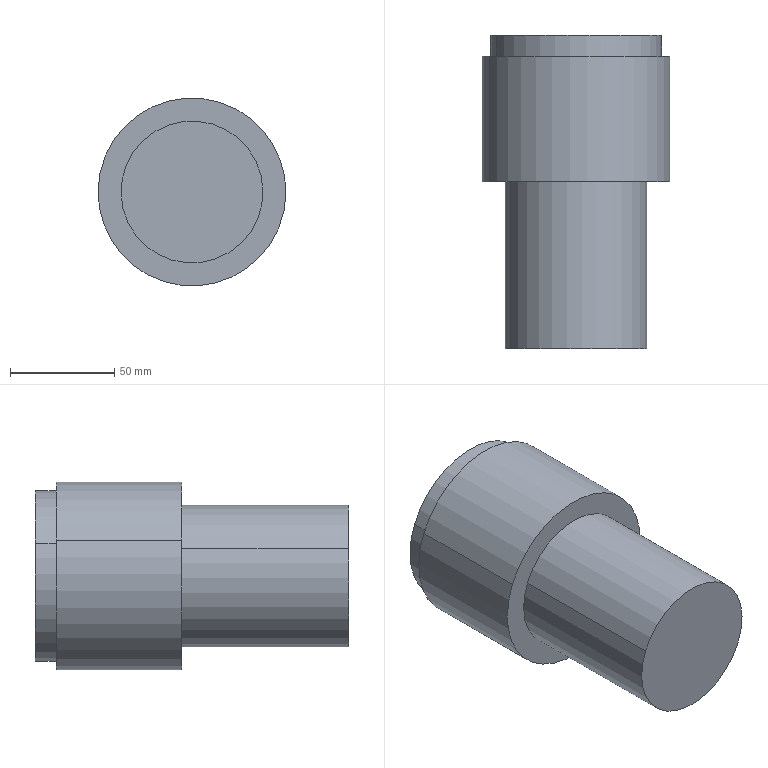Part | STEP file | Input 1-7 | 1 solid | 13 faces | box 90 x 150 x 90 mm | volume 629622 mm3 | cylinder 8 | plane 5 | commonest cylinder face diameters 45 x2 68 x2 82 x2 90 x2
STEP:
#1=CARTESIAN_POINT('',(-780.266,1724.418,3185.365));
#2=VERTEX_POINT('',#1);
#3=CARTESIAN_POINT('',(-717.452,1724.418,3159.318));
#4=VERTEX_POINT('',#3);
#5=CARTESIAN_POINT('',(-748.859,1724.418,3172.342));
#6=DIRECTION('',(0.,-1.,0.));
#7=DIRECTION('',(-0.9237,0.,0.383));
#8=AXIS2_PLACEMENT_3D('',#5,#6,#7);
#9=CIRCLE('',#8,34.);
#10=EDGE_CURVE('',#2,#4,#9,.T.);
#11=ORIENTED_EDGE('',*,*,#10,.F.);
#12=CARTESIAN_POINT('',(-780.266,1804.418,3185.365));
#13=VERTEX_POINT('',#12);
#14=CARTESIAN_POINT('',(-780.266,1724.418,3185.365));
#15=DIRECTION('',(0.,-1.,0.));
#16=VECTOR('',#15,1000.);
#17=LINE('',#14,#16);
#18=EDGE_CURVE('',#13,#2,#17,.T.);
#19=ORIENTED_EDGE('',*,*,#18,.F.);
#20=CARTESIAN_POINT('',(-717.452,1804.418,3159.318));
#21=VERTEX_POINT('',#20);
#22=CARTESIAN_POINT('',(-748.859,1804.418,3172.342));
#23=DIRECTION('',(0.,-1.,0.));
#24=DIRECTION('',(-0.9237,0.,0.383));
#25=AXIS2_PLACEMENT_3D('',#22,#23,#24);
#26=CIRCLE('',#25,34.);
#27=EDGE_CURVE('',#13,#21,#26,.T.);
#28=ORIENTED_EDGE('',*,*,#27,.T.);
#29=CARTESIAN_POINT('',(-717.452,1724.418,3159.318));
#30=DIRECTION('',(0.,-1.,0.));
#31=VECTOR('',#30,1000.);
#32=LINE('',#29,#31);
#33=EDGE_CURVE('',#21,#4,#32,.T.);
#34=ORIENTED_EDGE('',*,*,#33,.T.);
#35=EDGE_LOOP('',(#11,#19,#28,#34));
#36=FACE_OUTER_BOUND('',#35,.T.);
#37=CARTESIAN_POINT('',(-748.859,1724.418,3172.342));
#38=DIRECTION('',(0.,1.,0.));
#39=DIRECTION('',(-0.9237,0.,0.383));
#40=AXIS2_PLACEMENT_3D('',#37,#38,#39);
#41=CYLINDRICAL_SURFACE('',#40,34.);
#42=ADVANCED_FACE('',(#36),#41,.T.);
#43=CARTESIAN_POINT('',(-769.643,1814.418,3180.96));
#44=VERTEX_POINT('',#43);
#45=CARTESIAN_POINT('',(-728.075,1814.418,3163.723));
#46=VERTEX_POINT('',#45);
#47=CARTESIAN_POINT('',(-748.859,1814.418,3172.342));
#48=DIRECTION('',(0.,1.,0.));
#49=DIRECTION('',(-0.9237,0.,0.383));
#50=AXIS2_PLACEMENT_3D('',#47,#48,#49);
#51=CIRCLE('',#50,22.5);
#52=EDGE_CURVE('',#44,#46,#51,.T.);
#53=ORIENTED_EDGE('',*,*,#52,.F.);
#54=CARTESIAN_POINT('',(-769.643,1874.418,3180.96));
#55=VERTEX_POINT('',#54);
#56=CARTESIAN_POINT('',(-769.643,1724.418,3180.96));
#57=DIRECTION('',(0.,-1.,0.));
#58=VECTOR('',#57,1000.);
#59=LINE('',#56,#58);
#60=EDGE_CURVE('',#55,#44,#59,.T.);
#61=ORIENTED_EDGE('',*,*,#60,.F.);
#62=CARTESIAN_POINT('',(-728.075,1874.418,3163.723));
#63=VERTEX_POINT('',#62);
#64=CARTESIAN_POINT('',(-748.859,1874.418,3172.342));
#65=DIRECTION('',(0.,1.,0.));
#66=DIRECTION('',(0.9237,0.,-0.383));
#67=AXIS2_PLACEMENT_3D('',#64,#65,#66);
#68=CIRCLE('',#67,22.5);
#69=EDGE_CURVE('',#55,#63,#68,.T.);
#70=ORIENTED_EDGE('',*,*,#69,.T.);
#71=CARTESIAN_POINT('',(-728.075,1724.418,3163.723));
#72=DIRECTION('',(0.,-1.,0.));
#73=VECTOR('',#72,1000.);
#74=LINE('',#71,#73);
#75=EDGE_CURVE('',#63,#46,#74,.T.);
#76=ORIENTED_EDGE('',*,*,#75,.T.);
#77=EDGE_LOOP('',(#53,#61,#70,#76));
#78=FACE_OUTER_BOUND('',#77,.T.);
#79=CARTESIAN_POINT('',(-748.859,1724.418,3172.342));
#80=DIRECTION('',(0.,1.,0.));
#81=DIRECTION('',(-0.9237,0.,0.383));
#82=AXIS2_PLACEMENT_3D('',#79,#80,#81);
#83=CYLINDRICAL_SURFACE('',#82,22.5);
#84=ADVANCED_FACE('',(#78),#83,.F.);
#85=CARTESIAN_POINT('',(-710.986,1874.418,3156.637));
#86=VERTEX_POINT('',#85);
#87=CARTESIAN_POINT('',(-786.732,1874.418,3188.047));
#88=VERTEX_POINT('',#87);
#89=CARTESIAN_POINT('',(-748.859,1874.418,3172.342));
#90=DIRECTION('',(0.,1.,0.));
#91=DIRECTION('',(0.9237,0.,-0.383));
#92=AXIS2_PLACEMENT_3D('',#89,#90,#91);
#93=CIRCLE('',#92,41.);
#94=EDGE_CURVE('',#86,#88,#93,.T.);
#95=ORIENTED_EDGE('',*,*,#94,.F.);
#96=CARTESIAN_POINT('',(-710.986,1864.418,3156.637));
#97=VERTEX_POINT('',#96);
#98=CARTESIAN_POINT('',(-710.986,1874.418,3156.637));
#99=DIRECTION('',(0.,-1.,0.));
#100=VECTOR('',#99,1000.);
#101=LINE('',#98,#100);
#102=EDGE_CURVE('',#86,#97,#101,.T.);
#103=ORIENTED_EDGE('',*,*,#102,.T.);
#104=CARTESIAN_POINT('',(-786.732,1864.418,3188.047));
#105=VERTEX_POINT('',#104);
#106=CARTESIAN_POINT('',(-748.859,1864.418,3172.342));
#107=DIRECTION('',(0.,1.,0.));
#108=DIRECTION('',(-0.9237,0.,0.383));
#109=AXIS2_PLACEMENT_3D('',#106,#107,#108);
#110=CIRCLE('',#109,41.);
#111=EDGE_CURVE('',#97,#105,#110,.T.);
#112=ORIENTED_EDGE('',*,*,#111,.T.);
#113=CARTESIAN_POINT('',(-786.732,1874.418,3188.047));
#114=DIRECTION('',(0.,-1.,0.));
#115=VECTOR('',#114,1000.);
#116=LINE('',#113,#115);
#117=EDGE_CURVE('',#88,#105,#116,.T.);
#118=ORIENTED_EDGE('',*,*,#117,.F.);
#119=EDGE_LOOP('',(#95,#103,#112,#118));
#120=FACE_OUTER_BOUND('',#119,.T.);
#121=CARTESIAN_POINT('',(-748.859,1874.418,3172.342));
#122=DIRECTION('',(0.,-1.,0.));
#123=DIRECTION('',(0.9237,0.,-0.383));
#124=AXIS2_PLACEMENT_3D('',#121,#122,#123);
#125=CYLINDRICAL_SURFACE('',#124,41.);
#126=ADVANCED_FACE('',(#120),#125,.T.);
#127=CARTESIAN_POINT('',(-790.427,1804.418,3189.579));
#128=VERTEX_POINT('',#127);
#129=CARTESIAN_POINT('',(-707.291,1804.418,3155.105));
#130=VERTEX_POINT('',#129);
#131=CARTESIAN_POINT('',(-748.859,1804.418,3172.342));
#132=DIRECTION('',(0.,-1.,0.));
#133=DIRECTION('',(-0.9237,0.,0.383));
#134=AXIS2_PLACEMENT_3D('',#131,#132,#133);
#135=CIRCLE('',#134,45.);
#136=EDGE_CURVE('',#128,#130,#135,.T.);
#137=ORIENTED_EDGE('',*,*,#136,.F.);
#138=CARTESIAN_POINT('',(-790.427,1864.418,3189.579));
#139=VERTEX_POINT('',#138);
#140=CARTESIAN_POINT('',(-790.427,1814.418,3189.579));
#141=DIRECTION('',(0.,-1.,0.));
#142=VECTOR('',#141,1000.);
#143=LINE('',#140,#142);
#144=EDGE_CURVE('',#139,#128,#143,.T.);
#145=ORIENTED_EDGE('',*,*,#144,.F.);
#146=CARTESIAN_POINT('',(-707.291,1864.418,3155.105));
#147=VERTEX_POINT('',#146);
#148=CARTESIAN_POINT('',(-748.859,1864.418,3172.342));
#149=DIRECTION('',(0.,-1.,0.));
#150=DIRECTION('',(-0.9237,0.,0.383));
#151=AXIS2_PLACEMENT_3D('',#148,#149,#150);
#152=CIRCLE('',#151,45.);
#153=EDGE_CURVE('',#139,#147,#152,.T.);
#154=ORIENTED_EDGE('',*,*,#153,.T.);
#155=CARTESIAN_POINT('',(-707.291,1814.418,3155.105));
#156=DIRECTION('',(0.,-1.,0.));
#157=VECTOR('',#156,1000.);
#158=LINE('',#155,#157);
#159=EDGE_CURVE('',#147,#130,#158,.T.);
#160=ORIENTED_EDGE('',*,*,#159,.T.);
#161=EDGE_LOOP('',(#137,#145,#154,#160));
#162=FACE_OUTER_BOUND('',#161,.T.);
#163=CARTESIAN_POINT('',(-748.859,1814.418,3172.342));
#164=DIRECTION('',(0.,1.,0.));
#165=DIRECTION('',(-0.9237,0.,0.383));
#166=AXIS2_PLACEMENT_3D('',#163,#164,#165);
#167=CYLINDRICAL_SURFACE('',#166,45.);
#168=ADVANCED_FACE('',(#162),#167,.T.);
#169=CARTESIAN_POINT('',(-748.859,1804.418,3172.342));
#170=DIRECTION('',(0.,-1.,0.));
#171=DIRECTION('',(-0.9237,0.,0.383));
#172=AXIS2_PLACEMENT_3D('',#169,#170,#171);
#173=CIRCLE('',#172,45.);
#174=EDGE_CURVE('',#130,#128,#173,.T.);
#175=ORIENTED_EDGE('',*,*,#174,.T.);
#176=ORIENTED_EDGE('',*,*,#136,.T.);
#177=EDGE_LOOP('',(#175,#176));
#178=FACE_OUTER_BOUND('',#177,.T.);
#179=CARTESIAN_POINT('',(-748.859,1804.418,3172.342));
#180=DIRECTION('',(0.,-1.,0.));
#181=DIRECTION('',(-0.9237,0.,0.383));
#182=AXIS2_PLACEMENT_3D('',#179,#180,#181);
#183=CIRCLE('',#182,34.);
#184=EDGE_CURVE('',#21,#13,#183,.T.);
#185=ORIENTED_EDGE('',*,*,#184,.F.);
#186=ORIENTED_EDGE('',*,*,#27,.F.);
#187=EDGE_LOOP('',(#185,#186));
#188=FACE_BOUND('',#187,.T.);
#189=CARTESIAN_POINT('',(-748.859,1804.418,3172.342));
#190=DIRECTION('',(0.,-1.,0.));
#191=DIRECTION('',(0.9237,0.,-0.383));
#192=AXIS2_PLACEMENT_3D('',#189,#190,#191);
#193=PLANE('',#192);
#194=ADVANCED_FACE('',(#178,#188),#193,.T.);
#195=CARTESIAN_POINT('',(-748.859,1864.418,3172.342));
#196=DIRECTION('',(0.,-1.,0.));
#197=DIRECTION('',(-0.9237,0.,0.383));
#198=AXIS2_PLACEMENT_3D('',#195,#196,#197);
#199=CIRCLE('',#198,45.);
#200=EDGE_CURVE('',#147,#139,#199,.T.);
#201=ORIENTED_EDGE('',*,*,#200,.F.);
#202=ORIENTED_EDGE('',*,*,#153,.F.);
#203=EDGE_LOOP('',(#201,#202));
#204=FACE_OUTER_BOUND('',#203,.T.);
#205=CARTESIAN_POINT('',(-748.859,1864.418,3172.342));
#206=DIRECTION('',(0.,1.,0.));
#207=DIRECTION('',(-0.9237,0.,0.383));
#208=AXIS2_PLACEMENT_3D('',#205,#206,#207);
#209=CIRCLE('',#208,41.);
#210=EDGE_CURVE('',#105,#97,#209,.T.);
#211=ORIENTED_EDGE('',*,*,#210,.F.);
#212=ORIENTED_EDGE('',*,*,#111,.F.);
#213=EDGE_LOOP('',(#211,#212));
#214=FACE_BOUND('',#213,.T.);
#215=CARTESIAN_POINT('',(-748.859,1864.418,3172.342));
#216=DIRECTION('',(0.,-1.,0.));
#217=DIRECTION('',(0.9237,0.,-0.383));
#218=AXIS2_PLACEMENT_3D('',#215,#216,#217);
#219=PLANE('',#218);
#220=ADVANCED_FACE('',(#204,#214),#219,.F.);
#221=ORIENTED_EDGE('',*,*,#144,.T.);
#222=ORIENTED_EDGE('',*,*,#174,.F.);
#223=ORIENTED_EDGE('',*,*,#159,.F.);
#224=ORIENTED_EDGE('',*,*,#200,.T.);
#225=EDGE_LOOP('',(#221,#222,#223,#224));
#226=FACE_OUTER_BOUND('',#225,.T.);
#227=CARTESIAN_POINT('',(-748.859,1814.418,3172.342));
#228=DIRECTION('',(0.,1.,0.));
#229=DIRECTION('',(-0.9237,0.,0.383));
#230=AXIS2_PLACEMENT_3D('',#227,#228,#229);
#231=CYLINDRICAL_SURFACE('',#230,45.);
#232=ADVANCED_FACE('',(#226),#231,.T.);
#233=ORIENTED_EDGE('',*,*,#102,.F.);
#234=CARTESIAN_POINT('',(-748.859,1874.418,3172.342));
#235=DIRECTION('',(0.,1.,0.));
#236=DIRECTION('',(0.9237,0.,-0.383));
#237=AXIS2_PLACEMENT_3D('',#234,#235,#236);
#238=CIRCLE('',#237,41.);
#239=EDGE_CURVE('',#88,#86,#238,.T.);
#240=ORIENTED_EDGE('',*,*,#239,.F.);
#241=ORIENTED_EDGE('',*,*,#117,.T.);
#242=ORIENTED_EDGE('',*,*,#210,.T.);
#243=EDGE_LOOP('',(#233,#240,#241,#242));
#244=FACE_OUTER_BOUND('',#243,.T.);
#245=CARTESIAN_POINT('',(-748.859,1874.418,3172.342));
#246=DIRECTION('',(0.,-1.,0.));
#247=DIRECTION('',(0.9237,0.,-0.383));
#248=AXIS2_PLACEMENT_3D('',#245,#246,#247);
#249=CYLINDRICAL_SURFACE('',#248,41.);
#250=ADVANCED_FACE('',(#244),#249,.T.);
#251=CARTESIAN_POINT('',(-748.859,1874.418,3172.342));
#252=DIRECTION('',(0.,1.,0.));
#253=DIRECTION('',(0.9237,0.,-0.383));
#254=AXIS2_PLACEMENT_3D('',#251,#252,#253);
#255=CIRCLE('',#254,22.5);
#256=EDGE_CURVE('',#63,#55,#255,.T.);
#257=ORIENTED_EDGE('',*,*,#256,.F.);
#258=ORIENTED_EDGE('',*,*,#69,.F.);
#259=EDGE_LOOP('',(#257,#258));
#260=FACE_BOUND('',#259,.T.);
#261=ORIENTED_EDGE('',*,*,#239,.T.);
#262=ORIENTED_EDGE('',*,*,#94,.T.);
#263=EDGE_LOOP('',(#261,#262));
#264=FACE_OUTER_BOUND('',#263,.T.);
#265=CARTESIAN_POINT('',(-748.859,1874.418,3172.342));
#266=DIRECTION('',(0.,1.,0.));
#267=DIRECTION('',(-0.9237,0.,0.383));
#268=AXIS2_PLACEMENT_3D('',#265,#266,#267);
#269=PLANE('',#268);
#270=ADVANCED_FACE('',(#260,#264),#269,.T.);
#271=ORIENTED_EDGE('',*,*,#60,.T.);
#272=CARTESIAN_POINT('',(-748.859,1814.418,3172.342));
#273=DIRECTION('',(0.,1.,0.));
#274=DIRECTION('',(-0.9237,0.,0.383));
#275=AXIS2_PLACEMENT_3D('',#272,#273,#274);
#276=CIRCLE('',#275,22.5);
#277=EDGE_CURVE('',#46,#44,#276,.T.);
#278=ORIENTED_EDGE('',*,*,#277,.F.);
#279=ORIENTED_EDGE('',*,*,#75,.F.);
#280=ORIENTED_EDGE('',*,*,#256,.T.);
#281=EDGE_LOOP('',(#271,#278,#279,#280));
#282=FACE_OUTER_BOUND('',#281,.T.);
#283=CARTESIAN_POINT('',(-748.859,1724.418,3172.342));
#284=DIRECTION('',(0.,1.,0.));
#285=DIRECTION('',(-0.9237,0.,0.383));
#286=AXIS2_PLACEMENT_3D('',#283,#284,#285);
#287=CYLINDRICAL_SURFACE('',#286,22.5);
#288=ADVANCED_FACE('',(#282),#287,.F.);
#289=ORIENTED_EDGE('',*,*,#277,.T.);
#290=ORIENTED_EDGE('',*,*,#52,.T.);
#291=EDGE_LOOP('',(#289,#290));
#292=FACE_OUTER_BOUND('',#291,.T.);
#293=CARTESIAN_POINT('',(-748.859,1814.418,3172.342));
#294=DIRECTION('',(0.,-1.,0.));
#295=DIRECTION('',(0.9237,0.,-0.383));
#296=AXIS2_PLACEMENT_3D('',#293,#294,#295);
#297=PLANE('',#296);
#298=ADVANCED_FACE('',(#292),#297,.F.);
#299=ORIENTED_EDGE('',*,*,#18,.T.);
#300=CARTESIAN_POINT('',(-748.859,1724.418,3172.342));
#301=DIRECTION('',(0.,-1.,0.));
#302=DIRECTION('',(-0.9237,0.,0.383));
#303=AXIS2_PLACEMENT_3D('',#300,#301,#302);
#304=CIRCLE('',#303,34.);
#305=EDGE_CURVE('',#4,#2,#304,.T.);
#306=ORIENTED_EDGE('',*,*,#305,.F.);
#307=ORIENTED_EDGE('',*,*,#33,.F.);
#308=ORIENTED_EDGE('',*,*,#184,.T.);
#309=EDGE_LOOP('',(#299,#306,#307,#308));
#310=FACE_OUTER_BOUND('',#309,.T.);
#311=CARTESIAN_POINT('',(-748.859,1724.418,3172.342));
#312=DIRECTION('',(0.,1.,0.));
#313=DIRECTION('',(-0.9237,0.,0.383));
#314=AXIS2_PLACEMENT_3D('',#311,#312,#313);
#315=CYLINDRICAL_SURFACE('',#314,34.);
#316=ADVANCED_FACE('',(#310),#315,.T.);
#317=ORIENTED_EDGE('',*,*,#305,.T.);
#318=ORIENTED_EDGE('',*,*,#10,.T.);
#319=EDGE_LOOP('',(#317,#318));
#320=FACE_OUTER_BOUND('',#319,.T.);
#321=CARTESIAN_POINT('',(-748.859,1724.418,3172.342));
#322=DIRECTION('',(0.,-1.,0.));
#323=DIRECTION('',(0.9237,0.,-0.383));
#324=AXIS2_PLACEMENT_3D('',#321,#322,#323);
#325=PLANE('',#324);
#326=ADVANCED_FACE('',(#320),#325,.T.);
#327=CLOSED_SHELL('',(#42,#84,#126,#168,#194,#220,#232,#250,#270,#288,#298,#316,#326));
#328=MANIFOLD_SOLID_BREP('',#327);
#329=CARTESIAN_POINT('',(0.,0.,0.));
#330=DIRECTION('',(0.,0.,1.));
#331=DIRECTION('',(1.,0.,0.));
#332=AXIS2_PLACEMENT_3D('',#329,#330,#331);
#333=(LENGTH_UNIT()NAMED_UNIT(*)SI_UNIT(.MILLI.,.METRE.));
#334=UNCERTAINTY_MEASURE_WITH_UNIT(LENGTH_MEASURE(0.00001),#333,'','');
#335=(NAMED_UNIT(*)PLANE_ANGLE_UNIT()SI_UNIT($,.RADIAN.));
#336=(NAMED_UNIT(*)SI_UNIT($,.STERADIAN.)SOLID_ANGLE_UNIT());
#337=(GEOMETRIC_REPRESENTATION_CONTEXT(3)GLOBAL_UNCERTAINTY_ASSIGNED_CONTEXT((#334))GLOBAL_UNIT_ASSIGNED_CONTEXT((#333,#335,#336))REPRESENTATION_CONTEXT('',''));
#338=ADVANCED_BREP_SHAPE_REPRESENTATION('',(#328,#332),#337);